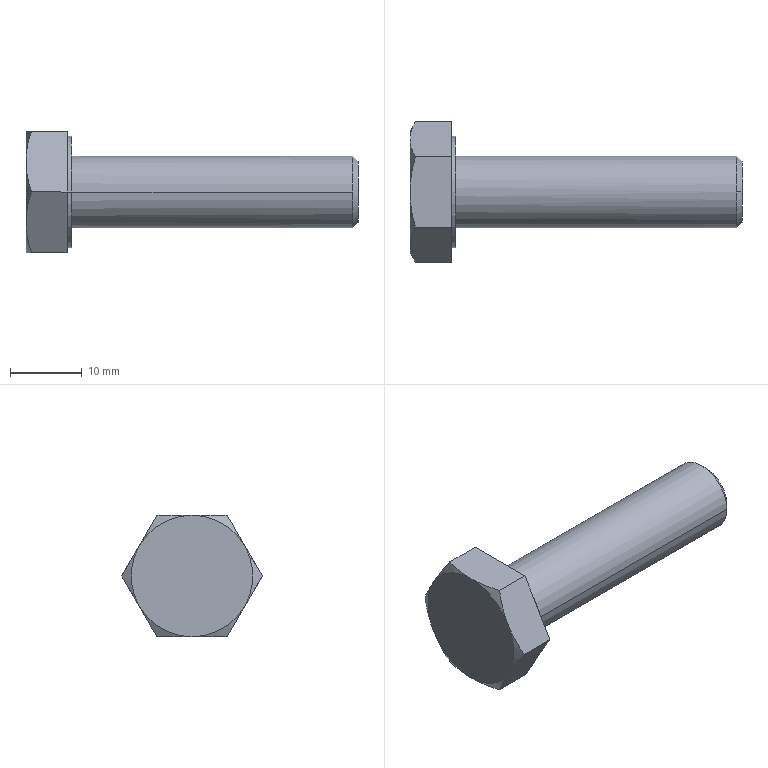Part | STEP file | DIN 960 - replaced by DIN EN 28765 M10 x 1.25 x 40 | 1 solid | 22 faces | box 46.4 x 19.63 x 17 mm | volume 4694 mm3 | plane 10 | cone 8 | cylinder 4 | commonest cylinder face diameters 10 x2 15.6 x2